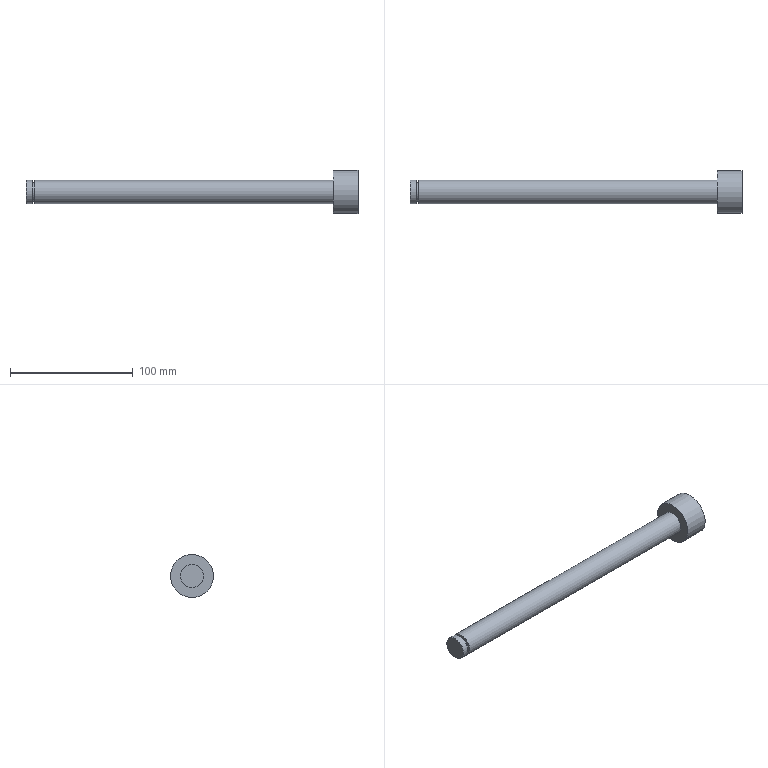Part | STEP file | SN10_002_005_FUSO | 1 solid | 9 faces | box 270 x 35 x 35 mm | volume 89911 mm3 | plane 5 | cylinder 4 | commonest cylinder face diameters 19 x2 15 x1 35 x1
STEP:
#1=CARTESIAN_POINT('',(0.,0.,0.));
#2=DIRECTION('',(0.,0.,1.));
#3=DIRECTION('',(1.,0.,0.));
#4=AXIS2_PLACEMENT_3D('',#1,#2,#3);
#5=CARTESIAN_POINT('',(140.,217.195,8.337));
#6=VERTEX_POINT('',#5);
#7=CARTESIAN_POINT('',(140.,221.75,0.));
#8=DIRECTION('',(1.,0.,0.));
#9=DIRECTION('',(0.,1.,0.));
#10=AXIS2_PLACEMENT_3D('',#7,#8,#9);
#11=CIRCLE('',#10,9.5);
#12=CARTESIAN_POINT('',(275.,221.75,0.));
#13=DIRECTION('',(1.,0.,0.));
#14=DIRECTION('',(0.,-0.4794,0.8776));
#15=AXIS2_PLACEMENT_3D('',#12,#13,#14);
#16=CYLINDRICAL_SURFACE('',#15,9.5);
#17=CARTESIAN_POINT('',(-2.071,-135.));
#18=DIRECTION('',(1.,0.));
#19=VECTOR('',#18,1.);
#20=LINE('',#17,#19);
#21=(GEOMETRIC_REPRESENTATION_CONTEXT(2)PARAMETRIC_REPRESENTATION_CONTEXT()REPRESENTATION_CONTEXT('',''));
#22=DEFINITIONAL_REPRESENTATION('',(#20),#21);
#23=PCURVE('',#16,#22);
#24=CARTESIAN_POINT('',(140.,221.75,9.5));
#25=DIRECTION('',(1.,0.,0.));
#26=DIRECTION('',(0.,0.,-1.));
#27=AXIS2_PLACEMENT_3D('',#24,#25,#26);
#28=PLANE('',#27);
#29=CARTESIAN_POINT('',(9.5,0.));
#30=DIRECTION('',(0.,1.));
#31=AXIS2_PLACEMENT_2D('',#29,#30);
#32=CIRCLE('',#31,9.5);
#33=(GEOMETRIC_REPRESENTATION_CONTEXT(2)PARAMETRIC_REPRESENTATION_CONTEXT()REPRESENTATION_CONTEXT('',''));
#34=DEFINITIONAL_REPRESENTATION('',(#32),#33);
#35=PCURVE('',#28,#34);
#36=SURFACE_CURVE('',#11,(#23,#35),.PCURVE_S1.);
#37=EDGE_CURVE('',#6,#6,#36,.T.);
#38=ORIENTED_EDGE('',*,*,#37,.T.);
#39=CARTESIAN_POINT('',(145.,217.195,8.337));
#40=VERTEX_POINT('',#39);
#41=CARTESIAN_POINT('',(140.,217.195,8.337));
#42=CARTESIAN_POINT('',(145.,217.195,8.337));
#43=B_SPLINE_CURVE_WITH_KNOTS('',1,(#41,#42),.UNSPECIFIED.,.F.,.F.,(2,2),(-135.,-130.),.PIECEWISE_BEZIER_KNOTS.);
#44=CARTESIAN_POINT('',(6.283,0.));
#45=DIRECTION('',(0.,1.));
#46=VECTOR('',#45,1.);
#47=LINE('',#44,#46);
#48=(GEOMETRIC_REPRESENTATION_CONTEXT(2)PARAMETRIC_REPRESENTATION_CONTEXT()REPRESENTATION_CONTEXT('',''));
#49=DEFINITIONAL_REPRESENTATION('',(#47),#48);
#50=PCURVE('',#16,#49);
#51=CARTESIAN_POINT('',(0.,0.));
#52=DIRECTION('',(0.,1.));
#53=VECTOR('',#52,1.);
#54=LINE('',#51,#53);
#55=(GEOMETRIC_REPRESENTATION_CONTEXT(2)PARAMETRIC_REPRESENTATION_CONTEXT()REPRESENTATION_CONTEXT('',''));
#56=DEFINITIONAL_REPRESENTATION('',(#54),#55);
#57=PCURVE('',#16,#56);
#58=SEAM_CURVE('',#43,(#50,#57),.PCURVE_S1.);
#59=EDGE_CURVE('',#6,#40,#58,.T.);
#60=ORIENTED_EDGE('',*,*,#59,.T.);
#61=CARTESIAN_POINT('',(145.,221.75,0.));
#62=DIRECTION('',(1.,0.,0.));
#63=DIRECTION('',(0.,1.,0.));
#64=AXIS2_PLACEMENT_3D('',#61,#62,#63);
#65=CIRCLE('',#64,9.5);
#66=CARTESIAN_POINT('',(-2.071,-130.));
#67=DIRECTION('',(1.,0.));
#68=VECTOR('',#67,1.);
#69=LINE('',#66,#68);
#70=(GEOMETRIC_REPRESENTATION_CONTEXT(2)PARAMETRIC_REPRESENTATION_CONTEXT()REPRESENTATION_CONTEXT('',''));
#71=DEFINITIONAL_REPRESENTATION('',(#69),#70);
#72=PCURVE('',#16,#71);
#73=CARTESIAN_POINT('',(145.,221.75,7.5));
#74=DIRECTION('',(1.,0.,0.));
#75=DIRECTION('',(0.,0.,-1.));
#76=AXIS2_PLACEMENT_3D('',#73,#74,#75);
#77=PLANE('',#76);
#78=CARTESIAN_POINT('',(7.5,0.));
#79=DIRECTION('',(0.,1.));
#80=AXIS2_PLACEMENT_2D('',#78,#79);
#81=CIRCLE('',#80,9.5);
#82=(GEOMETRIC_REPRESENTATION_CONTEXT(2)PARAMETRIC_REPRESENTATION_CONTEXT()REPRESENTATION_CONTEXT('',''));
#83=DEFINITIONAL_REPRESENTATION('',(#81),#82);
#84=PCURVE('',#77,#83);
#85=SURFACE_CURVE('',#65,(#72,#84),.PCURVE_S1.);
#86=EDGE_CURVE('',#40,#40,#85,.T.);
#87=ORIENTED_EDGE('',*,*,#86,.F.);
#88=ORIENTED_EDGE('',*,*,#59,.F.);
#89=EDGE_LOOP('',(#38,#60,#87,#88));
#90=FACE_BOUND('',#89,.T.);
#91=ADVANCED_FACE('',(#90),#16,.T.);
#92=CARTESIAN_POINT('',(145.,218.154,6.582));
#93=VERTEX_POINT('',#92);
#94=CARTESIAN_POINT('',(145.,221.75,0.));
#95=DIRECTION('',(1.,0.,0.));
#96=DIRECTION('',(0.,1.,0.));
#97=AXIS2_PLACEMENT_3D('',#94,#95,#96);
#98=CIRCLE('',#97,7.5);
#99=CARTESIAN_POINT('',(275.,221.75,0.));
#100=DIRECTION('',(1.,0.,0.));
#101=DIRECTION('',(0.,-0.4794,0.8776));
#102=AXIS2_PLACEMENT_3D('',#99,#100,#101);
#103=CYLINDRICAL_SURFACE('',#102,7.5);
#104=CARTESIAN_POINT('',(-2.071,-130.));
#105=DIRECTION('',(1.,0.));
#106=VECTOR('',#105,1.);
#107=LINE('',#104,#106);
#108=(GEOMETRIC_REPRESENTATION_CONTEXT(2)PARAMETRIC_REPRESENTATION_CONTEXT()REPRESENTATION_CONTEXT('',''));
#109=DEFINITIONAL_REPRESENTATION('',(#107),#108);
#110=PCURVE('',#103,#109);
#111=CARTESIAN_POINT('',(7.5,0.));
#112=DIRECTION('',(0.,1.));
#113=AXIS2_PLACEMENT_2D('',#111,#112);
#114=CIRCLE('',#113,7.5);
#115=(GEOMETRIC_REPRESENTATION_CONTEXT(2)PARAMETRIC_REPRESENTATION_CONTEXT()REPRESENTATION_CONTEXT('',''));
#116=DEFINITIONAL_REPRESENTATION('',(#114),#115);
#117=PCURVE('',#77,#116);
#118=SURFACE_CURVE('',#98,(#110,#117),.PCURVE_S1.);
#119=EDGE_CURVE('',#93,#93,#118,.T.);
#120=ORIENTED_EDGE('',*,*,#119,.T.);
#121=CARTESIAN_POINT('',(147.,218.154,6.582));
#122=VERTEX_POINT('',#121);
#123=CARTESIAN_POINT('',(145.,218.154,6.582));
#124=CARTESIAN_POINT('',(147.,218.154,6.582));
#125=B_SPLINE_CURVE_WITH_KNOTS('',1,(#123,#124),.UNSPECIFIED.,.F.,.F.,(2,2),(-130.,-128.),.PIECEWISE_BEZIER_KNOTS.);
#126=CARTESIAN_POINT('',(6.283,0.));
#127=DIRECTION('',(0.,1.));
#128=VECTOR('',#127,1.);
#129=LINE('',#126,#128);
#130=(GEOMETRIC_REPRESENTATION_CONTEXT(2)PARAMETRIC_REPRESENTATION_CONTEXT()REPRESENTATION_CONTEXT('',''));
#131=DEFINITIONAL_REPRESENTATION('',(#129),#130);
#132=PCURVE('',#103,#131);
#133=CARTESIAN_POINT('',(0.,0.));
#134=DIRECTION('',(0.,1.));
#135=VECTOR('',#134,1.);
#136=LINE('',#133,#135);
#137=(GEOMETRIC_REPRESENTATION_CONTEXT(2)PARAMETRIC_REPRESENTATION_CONTEXT()REPRESENTATION_CONTEXT('',''));
#138=DEFINITIONAL_REPRESENTATION('',(#136),#137);
#139=PCURVE('',#103,#138);
#140=SEAM_CURVE('',#125,(#132,#139),.PCURVE_S1.);
#141=EDGE_CURVE('',#93,#122,#140,.T.);
#142=ORIENTED_EDGE('',*,*,#141,.T.);
#143=CARTESIAN_POINT('',(147.,221.75,0.));
#144=DIRECTION('',(1.,0.,0.));
#145=DIRECTION('',(0.,1.,0.));
#146=AXIS2_PLACEMENT_3D('',#143,#144,#145);
#147=CIRCLE('',#146,7.5);
#148=CARTESIAN_POINT('',(-2.071,-128.));
#149=DIRECTION('',(1.,0.));
#150=VECTOR('',#149,1.);
#151=LINE('',#148,#150);
#152=(GEOMETRIC_REPRESENTATION_CONTEXT(2)PARAMETRIC_REPRESENTATION_CONTEXT()REPRESENTATION_CONTEXT('',''));
#153=DEFINITIONAL_REPRESENTATION('',(#151),#152);
#154=PCURVE('',#103,#153);
#155=CARTESIAN_POINT('',(147.,221.75,9.5));
#156=DIRECTION('',(1.,0.,0.));
#157=DIRECTION('',(0.,0.,-1.));
#158=AXIS2_PLACEMENT_3D('',#155,#156,#157);
#159=PLANE('',#158);
#160=CARTESIAN_POINT('',(9.5,0.));
#161=DIRECTION('',(0.,1.));
#162=AXIS2_PLACEMENT_2D('',#160,#161);
#163=CIRCLE('',#162,7.5);
#164=(GEOMETRIC_REPRESENTATION_CONTEXT(2)PARAMETRIC_REPRESENTATION_CONTEXT()REPRESENTATION_CONTEXT('',''));
#165=DEFINITIONAL_REPRESENTATION('',(#163),#164);
#166=PCURVE('',#159,#165);
#167=SURFACE_CURVE('',#147,(#154,#166),.PCURVE_S1.);
#168=EDGE_CURVE('',#122,#122,#167,.T.);
#169=ORIENTED_EDGE('',*,*,#168,.F.);
#170=ORIENTED_EDGE('',*,*,#141,.F.);
#171=EDGE_LOOP('',(#120,#142,#169,#170));
#172=FACE_BOUND('',#171,.T.);
#173=ADVANCED_FACE('',(#172),#103,.T.);
#174=CARTESIAN_POINT('',(147.,217.195,8.337));
#175=VERTEX_POINT('',#174);
#176=CARTESIAN_POINT('',(147.,221.75,0.));
#177=DIRECTION('',(1.,0.,0.));
#178=DIRECTION('',(0.,1.,0.));
#179=AXIS2_PLACEMENT_3D('',#176,#177,#178);
#180=CIRCLE('',#179,9.5);
#181=CARTESIAN_POINT('',(275.,221.75,0.));
#182=DIRECTION('',(1.,0.,0.));
#183=DIRECTION('',(0.,-0.4794,0.8776));
#184=AXIS2_PLACEMENT_3D('',#181,#182,#183);
#185=CYLINDRICAL_SURFACE('',#184,9.5);
#186=CARTESIAN_POINT('',(-2.071,-128.));
#187=DIRECTION('',(1.,0.));
#188=VECTOR('',#187,1.);
#189=LINE('',#186,#188);
#190=(GEOMETRIC_REPRESENTATION_CONTEXT(2)PARAMETRIC_REPRESENTATION_CONTEXT()REPRESENTATION_CONTEXT('',''));
#191=DEFINITIONAL_REPRESENTATION('',(#189),#190);
#192=PCURVE('',#185,#191);
#193=CARTESIAN_POINT('',(9.5,0.));
#194=DIRECTION('',(0.,1.));
#195=AXIS2_PLACEMENT_2D('',#193,#194);
#196=CIRCLE('',#195,9.5);
#197=(GEOMETRIC_REPRESENTATION_CONTEXT(2)PARAMETRIC_REPRESENTATION_CONTEXT()REPRESENTATION_CONTEXT('',''));
#198=DEFINITIONAL_REPRESENTATION('',(#196),#197);
#199=PCURVE('',#159,#198);
#200=SURFACE_CURVE('',#180,(#192,#199),.PCURVE_S1.);
#201=EDGE_CURVE('',#175,#175,#200,.T.);
#202=ORIENTED_EDGE('',*,*,#201,.T.);
#203=CARTESIAN_POINT('',(390.,217.195,8.337));
#204=VERTEX_POINT('',#203);
#205=CARTESIAN_POINT('',(147.,217.195,8.337));
#206=CARTESIAN_POINT('',(390.,217.195,8.337));
#207=B_SPLINE_CURVE_WITH_KNOTS('',1,(#205,#206),.UNSPECIFIED.,.F.,.F.,(2,2),(-128.,115.),.PIECEWISE_BEZIER_KNOTS.);
#208=CARTESIAN_POINT('',(6.283,0.));
#209=DIRECTION('',(0.,1.));
#210=VECTOR('',#209,1.);
#211=LINE('',#208,#210);
#212=(GEOMETRIC_REPRESENTATION_CONTEXT(2)PARAMETRIC_REPRESENTATION_CONTEXT()REPRESENTATION_CONTEXT('',''));
#213=DEFINITIONAL_REPRESENTATION('',(#211),#212);
#214=PCURVE('',#185,#213);
#215=CARTESIAN_POINT('',(0.,0.));
#216=DIRECTION('',(0.,1.));
#217=VECTOR('',#216,1.);
#218=LINE('',#215,#217);
#219=(GEOMETRIC_REPRESENTATION_CONTEXT(2)PARAMETRIC_REPRESENTATION_CONTEXT()REPRESENTATION_CONTEXT('',''));
#220=DEFINITIONAL_REPRESENTATION('',(#218),#219);
#221=PCURVE('',#185,#220);
#222=SEAM_CURVE('',#207,(#214,#221),.PCURVE_S1.);
#223=EDGE_CURVE('',#175,#204,#222,.T.);
#224=ORIENTED_EDGE('',*,*,#223,.T.);
#225=CARTESIAN_POINT('',(390.,221.75,0.));
#226=DIRECTION('',(1.,0.,0.));
#227=DIRECTION('',(0.,1.,0.));
#228=AXIS2_PLACEMENT_3D('',#225,#226,#227);
#229=CIRCLE('',#228,9.5);
#230=CARTESIAN_POINT('',(-2.071,115.));
#231=DIRECTION('',(1.,0.));
#232=VECTOR('',#231,1.);
#233=LINE('',#230,#232);
#234=(GEOMETRIC_REPRESENTATION_CONTEXT(2)PARAMETRIC_REPRESENTATION_CONTEXT()REPRESENTATION_CONTEXT('',''));
#235=DEFINITIONAL_REPRESENTATION('',(#233),#234);
#236=PCURVE('',#185,#235);
#237=CARTESIAN_POINT('',(390.,221.75,17.5));
#238=DIRECTION('',(1.,0.,0.));
#239=DIRECTION('',(0.,0.,-1.));
#240=AXIS2_PLACEMENT_3D('',#237,#238,#239);
#241=PLANE('',#240);
#242=CARTESIAN_POINT('',(17.5,0.));
#243=DIRECTION('',(0.,1.));
#244=AXIS2_PLACEMENT_2D('',#242,#243);
#245=CIRCLE('',#244,9.5);
#246=(GEOMETRIC_REPRESENTATION_CONTEXT(2)PARAMETRIC_REPRESENTATION_CONTEXT()REPRESENTATION_CONTEXT('',''));
#247=DEFINITIONAL_REPRESENTATION('',(#245),#246);
#248=PCURVE('',#241,#247);
#249=SURFACE_CURVE('',#229,(#236,#248),.PCURVE_S1.);
#250=EDGE_CURVE('',#204,#204,#249,.T.);
#251=ORIENTED_EDGE('',*,*,#250,.F.);
#252=ORIENTED_EDGE('',*,*,#223,.F.);
#253=EDGE_LOOP('',(#202,#224,#251,#252));
#254=FACE_BOUND('',#253,.T.);
#255=ADVANCED_FACE('',(#254),#185,.T.);
#256=CARTESIAN_POINT('',(390.,213.36,15.358));
#257=VERTEX_POINT('',#256);
#258=CARTESIAN_POINT('',(390.,221.75,0.));
#259=DIRECTION('',(1.,0.,0.));
#260=DIRECTION('',(0.,1.,0.));
#261=AXIS2_PLACEMENT_3D('',#258,#259,#260);
#262=CIRCLE('',#261,17.5);
#263=CARTESIAN_POINT('',(275.,221.75,0.));
#264=DIRECTION('',(1.,0.,0.));
#265=DIRECTION('',(0.,-0.4794,0.8776));
#266=AXIS2_PLACEMENT_3D('',#263,#264,#265);
#267=CYLINDRICAL_SURFACE('',#266,17.5);
#268=CARTESIAN_POINT('',(-2.071,115.));
#269=DIRECTION('',(1.,0.));
#270=VECTOR('',#269,1.);
#271=LINE('',#268,#270);
#272=(GEOMETRIC_REPRESENTATION_CONTEXT(2)PARAMETRIC_REPRESENTATION_CONTEXT()REPRESENTATION_CONTEXT('',''));
#273=DEFINITIONAL_REPRESENTATION('',(#271),#272);
#274=PCURVE('',#267,#273);
#275=CARTESIAN_POINT('',(17.5,0.));
#276=DIRECTION('',(0.,1.));
#277=AXIS2_PLACEMENT_2D('',#275,#276);
#278=CIRCLE('',#277,17.5);
#279=(GEOMETRIC_REPRESENTATION_CONTEXT(2)PARAMETRIC_REPRESENTATION_CONTEXT()REPRESENTATION_CONTEXT('',''));
#280=DEFINITIONAL_REPRESENTATION('',(#278),#279);
#281=PCURVE('',#241,#280);
#282=SURFACE_CURVE('',#262,(#274,#281),.PCURVE_S1.);
#283=EDGE_CURVE('',#257,#257,#282,.T.);
#284=ORIENTED_EDGE('',*,*,#283,.T.);
#285=CARTESIAN_POINT('',(410.,213.36,15.358));
#286=VERTEX_POINT('',#285);
#287=CARTESIAN_POINT('',(390.,213.36,15.358));
#288=CARTESIAN_POINT('',(410.,213.36,15.358));
#289=B_SPLINE_CURVE_WITH_KNOTS('',1,(#287,#288),.UNSPECIFIED.,.F.,.F.,(2,2),(115.,135.),.PIECEWISE_BEZIER_KNOTS.);
#290=CARTESIAN_POINT('',(6.283,0.));
#291=DIRECTION('',(0.,1.));
#292=VECTOR('',#291,1.);
#293=LINE('',#290,#292);
#294=(GEOMETRIC_REPRESENTATION_CONTEXT(2)PARAMETRIC_REPRESENTATION_CONTEXT()REPRESENTATION_CONTEXT('',''));
#295=DEFINITIONAL_REPRESENTATION('',(#293),#294);
#296=PCURVE('',#267,#295);
#297=CARTESIAN_POINT('',(0.,0.));
#298=DIRECTION('',(0.,1.));
#299=VECTOR('',#298,1.);
#300=LINE('',#297,#299);
#301=(GEOMETRIC_REPRESENTATION_CONTEXT(2)PARAMETRIC_REPRESENTATION_CONTEXT()REPRESENTATION_CONTEXT('',''));
#302=DEFINITIONAL_REPRESENTATION('',(#300),#301);
#303=PCURVE('',#267,#302);
#304=SEAM_CURVE('',#289,(#296,#303),.PCURVE_S1.);
#305=EDGE_CURVE('',#257,#286,#304,.T.);
#306=ORIENTED_EDGE('',*,*,#305,.T.);
#307=CARTESIAN_POINT('',(410.,221.75,0.));
#308=DIRECTION('',(1.,0.,0.));
#309=DIRECTION('',(0.,1.,0.));
#310=AXIS2_PLACEMENT_3D('',#307,#308,#309);
#311=CIRCLE('',#310,17.5);
#312=CARTESIAN_POINT('',(-2.071,135.));
#313=DIRECTION('',(1.,0.));
#314=VECTOR('',#313,1.);
#315=LINE('',#312,#314);
#316=(GEOMETRIC_REPRESENTATION_CONTEXT(2)PARAMETRIC_REPRESENTATION_CONTEXT()REPRESENTATION_CONTEXT('',''));
#317=DEFINITIONAL_REPRESENTATION('',(#315),#316);
#318=PCURVE('',#267,#317);
#319=CARTESIAN_POINT('',(410.,221.75,0.));
#320=DIRECTION('',(1.,0.,0.));
#321=DIRECTION('',(0.,0.,-1.));
#322=AXIS2_PLACEMENT_3D('',#319,#320,#321);
#323=PLANE('',#322);
#324=CARTESIAN_POINT('',(0.,0.));
#325=DIRECTION('',(0.,1.));
#326=AXIS2_PLACEMENT_2D('',#324,#325);
#327=CIRCLE('',#326,17.5);
#328=(GEOMETRIC_REPRESENTATION_CONTEXT(2)PARAMETRIC_REPRESENTATION_CONTEXT()REPRESENTATION_CONTEXT('',''));
#329=DEFINITIONAL_REPRESENTATION('',(#327),#328);
#330=PCURVE('',#323,#329);
#331=SURFACE_CURVE('',#311,(#318,#330),.PCURVE_S1.);
#332=EDGE_CURVE('',#286,#286,#331,.T.);
#333=ORIENTED_EDGE('',*,*,#332,.F.);
#334=ORIENTED_EDGE('',*,*,#305,.F.);
#335=EDGE_LOOP('',(#284,#306,#333,#334));
#336=FACE_BOUND('',#335,.T.);
#337=ADVANCED_FACE('',(#336),#267,.T.);
#338=ORIENTED_EDGE('',*,*,#37,.F.);
#339=EDGE_LOOP('',(#338));
#340=FACE_BOUND('',#339,.T.);
#341=ADVANCED_FACE('',(#340),#28,.F.);
#342=ORIENTED_EDGE('',*,*,#86,.T.);
#343=EDGE_LOOP('',(#342));
#344=FACE_BOUND('',#343,.T.);
#345=ORIENTED_EDGE('',*,*,#119,.F.);
#346=EDGE_LOOP('',(#345));
#347=FACE_BOUND('',#346,.T.);
#348=ADVANCED_FACE('',(#344,#347),#77,.T.);
#349=ORIENTED_EDGE('',*,*,#201,.F.);
#350=EDGE_LOOP('',(#349));
#351=FACE_BOUND('',#350,.T.);
#352=ORIENTED_EDGE('',*,*,#168,.T.);
#353=EDGE_LOOP('',(#352));
#354=FACE_BOUND('',#353,.T.);
#355=ADVANCED_FACE('',(#351,#354),#159,.F.);
#356=ORIENTED_EDGE('',*,*,#283,.F.);
#357=EDGE_LOOP('',(#356));
#358=FACE_BOUND('',#357,.T.);
#359=ORIENTED_EDGE('',*,*,#250,.T.);
#360=EDGE_LOOP('',(#359));
#361=FACE_BOUND('',#360,.T.);
#362=ADVANCED_FACE('',(#358,#361),#241,.F.);
#363=ORIENTED_EDGE('',*,*,#332,.T.);
#364=EDGE_LOOP('',(#363));
#365=FACE_BOUND('',#364,.T.);
#366=ADVANCED_FACE('',(#365),#323,.T.);
#367=CLOSED_SHELL('',(#91,#173,#255,#337,#341,#348,#355,#362,#366));
#368=MANIFOLD_SOLID_BREP('',#367);
#369=(LENGTH_UNIT()NAMED_UNIT(*)SI_UNIT(.MILLI.,.METRE.));
#370=UNCERTAINTY_MEASURE_WITH_UNIT(LENGTH_MEASURE(0.00001),#369,'','');
#371=(NAMED_UNIT(*)PLANE_ANGLE_UNIT()SI_UNIT($,.RADIAN.));
#372=(NAMED_UNIT(*)SI_UNIT($,.STERADIAN.)SOLID_ANGLE_UNIT());
#373=(GEOMETRIC_REPRESENTATION_CONTEXT(3)GLOBAL_UNCERTAINTY_ASSIGNED_CONTEXT((#370))GLOBAL_UNIT_ASSIGNED_CONTEXT((#369,#371,#372))REPRESENTATION_CONTEXT('',''));
#374=ADVANCED_BREP_SHAPE_REPRESENTATION('',(#4,#368),#373);